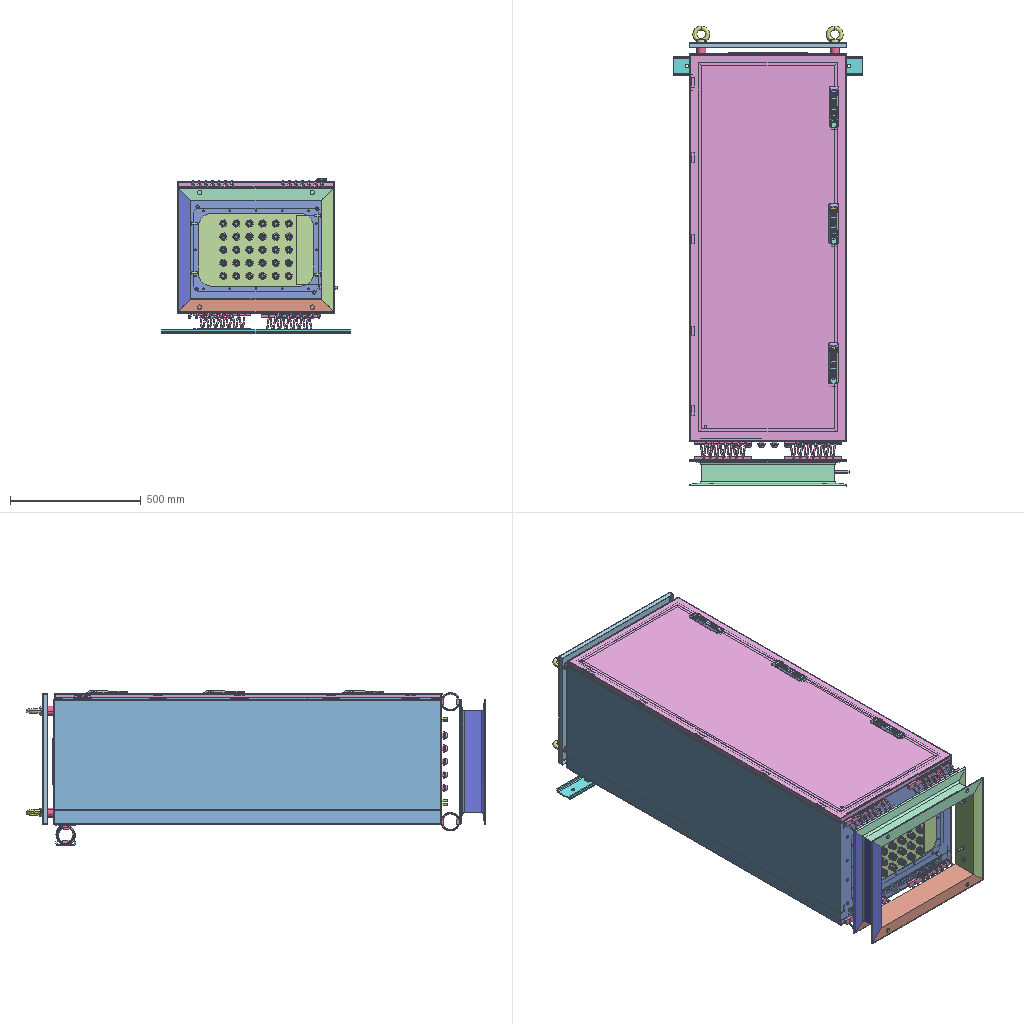Assembly | SolidWorks | 42 different items | 120 placed | box 720 x 1756 x 593 mm
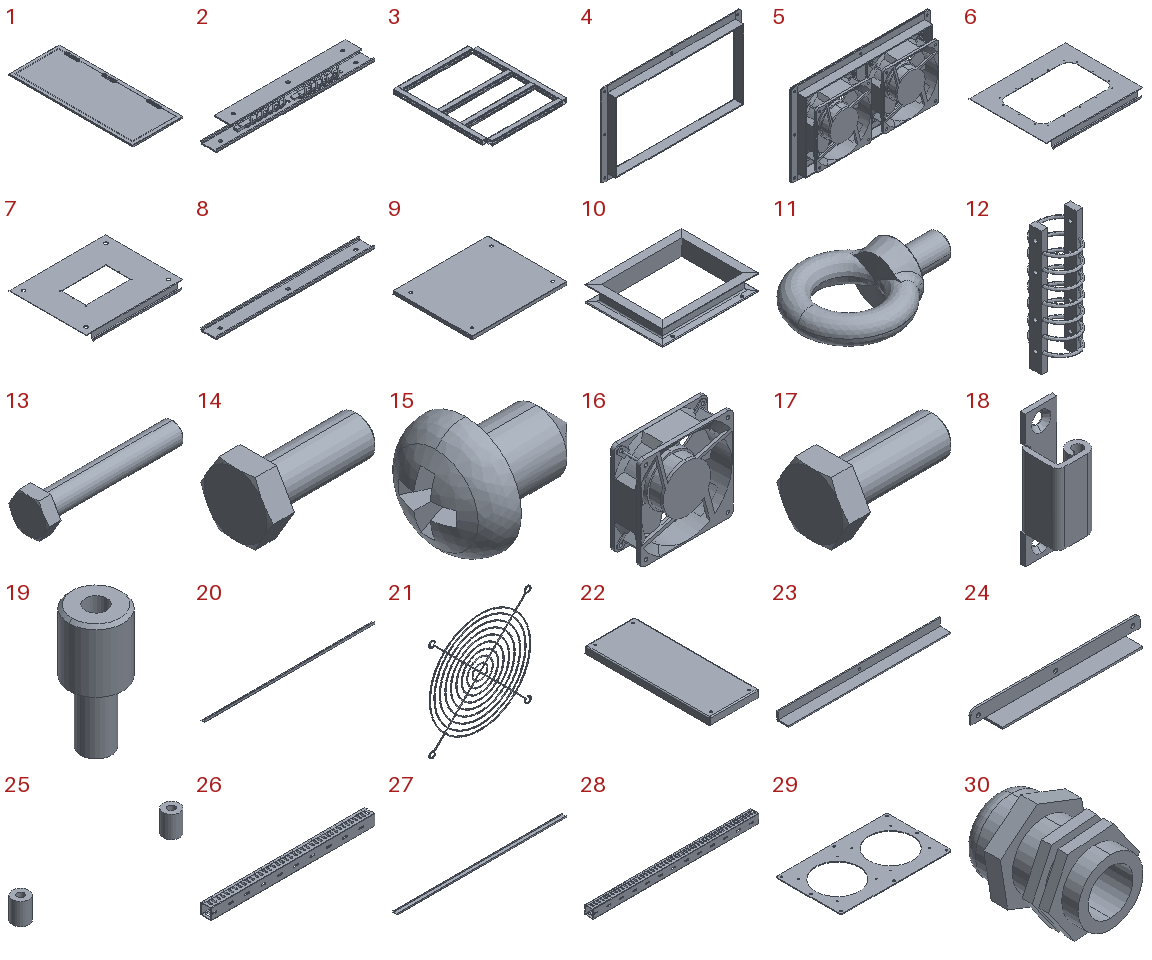Parts list (item | name | quantity | parent item | size | volume | features):
1 | (subassembly) | x1 | - | 599 x 1482 x 37.95 mm | 2644503 mm3 | -
2 | (subassembly) | x1 | - | 720 x 75 x 82.954 mm | 767649 mm3 | -
3 | (subassembly) | x1 | - | - | 575981 mm3 | -
4 | (subassembly) | x1 | in 5 | 300 x 20 x 176 mm | 55930 mm3 | -
5 | (subassembly) | x1 | - | 300 x 40.8 x 176 mm | 500898 mm3 | -
6 | - | x1 | - | 600 x 496 x 35 mm | 393982 mm3 | features MoveFace 2, BaseBody 1
7 | - | x1 | - | 600 x 496 x 35 mm | 549272 mm3 | features ICE 2, MoveFace 2, BaseBody 1
8 | - | x1 | in 2 | 720 x 75 x 15 mm | 322694 mm3 | features MoveFace 4, Fillet 2, BaseBody 1, ICE 1
9 | - | x1 | - | 600 x 500 x 20 mm | 675087 mm3 | features BaseBody 1, MoveFace 1
10 | - | x1 | - | 600 x 478 x 100 mm | 2451873 mm3 | features BaseBody 4, MoveCopyBody 2, MoveFace 2
11 | - | x4 | - | 91.2 x 64.4 x 35.09 mm | 39752 mm3 | features BaseBody 1
12 | - | x6 | in 2 | 71 x 70 x 216 mm | 111132 mm3 | features BaseBody 1, ICE 1
13 | - | x1 | - | 66.4 x 18.475 x 16 mm | 6099 mm3 | features BaseBody 1
14 | - | x1 | - | 18.975 x 11.258 x 9.75 mm | 741.836 mm3 | features BaseBody 1, MoveFace 1, Scale 1
15 | - | x6 | - | 14.243 x 11.05 x 11.056 mm | 485.827 mm3 | features BaseBody 1, MoveFace 1
16 | - | x2 | in 5 | 119.126 x 38.1 x 119.126 mm | 190423 mm3 | features BaseBody 1
17 | - | x8 | - | 25.3 x 15.011 x 13 mm | 1758 mm3 | features BaseBody 1, MoveFace 1
18 | - | x5 | - | 20 x 20 x 67 mm | 6811 mm3 | features BaseBody 1
19 | - | x4 | - | 35 x 35 x 80 mm | 47545 mm3 | features BaseBody 1
20 | - | x6 | - | 1472 x 31 x 20 mm | 172321 mm3 | features BaseBody 1, ICE 1, MoveFace 1
21 | - | x2 | in 5 | 111.7 x 0.7 x 111.7 mm | 1043 mm3 | features BaseBody 1
22 | - | x1 | - | 105 x 265 x 15 mm | 73841 mm3 | features BaseBody 1
23 | - | x2 | in 4 | 274 x 20 x 15 mm | 17798 mm3 | features BaseBody 1
24 | - | x2 | in 4 | 176 x 20 x 15 mm | 10168 mm3 | features BaseBody 1
25 | - | x2 | - | 122 x 12 x 16 mm | 3011 mm3 | features BaseBody 2
26 | - | x4 | in 3 | 502 x 31.5 x 34 mm | 88043 mm3 | features BaseBody 2, ICE 1
27 | - | x1 | - | 1475 x 40 x 12 mm | 174214 mm3 | features BaseBody 1, MoveFace 1
28 | - | x2 | in 3 | 640 x 31.5 x 34 mm | 111904 mm3 | features BaseBody 2
29 | - | x1 | in 5 | 300 x 176 x 2 mm | 62035 mm3 | features BaseBody 1
30 | - | x30 | - | 27.604 x 35 x 28.514 mm | 7936 mm3 | features ICE 5, Extrusion 1, Fillet 1, Shell 1
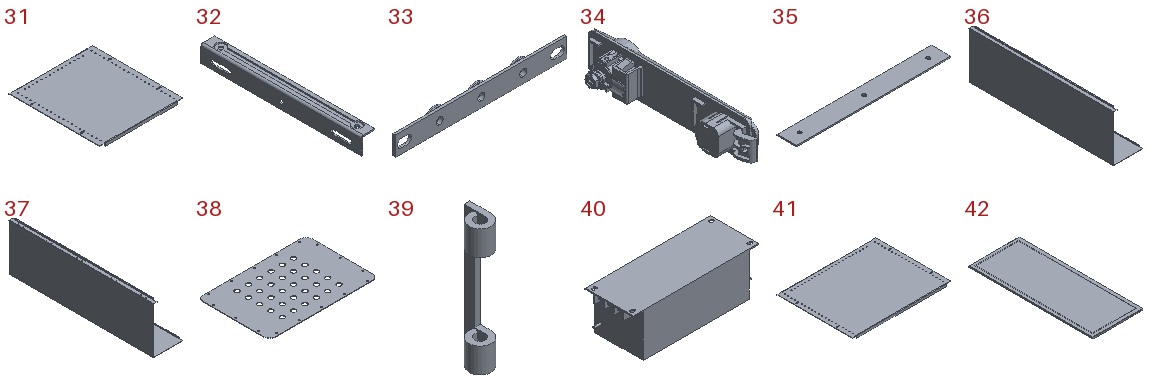31 | - | x6 | - | 406 x 440 x 15 mm | 372648 mm3 | features ICE 5, MoveFace 4, BaseBody 1
32 | - | x1 | - | 20 x 233 x 25 mm | 22029 mm3 | features ICE 4, Extrusion 1
33 | - | x2 | - | 123 x 4 x 15 mm | 4060 mm3 | features ICE 2, Extrusion 1
34 | - | x3 | in 1 | 37.95 x 165.2 x 36 mm | 54384 mm3 | features BaseBody 4
35 | - | x1 | in 2 | 600 x 75 x 5 mm | 222691 mm3 | features MoveFace 2, BaseBody 1
36 | - | x1 | - | 300 x 1476 x 496 mm | 2482636 mm3 | features ICE 3, MoveFace 3, BaseBody 1, Fillet 1
37 | - | x1 | - | 300 x 1476 x 496 mm | 2482160 mm3 | features MoveFace 6, ICE 3, BaseBody 1, Fillet 1
38 | - | x1 | - | 480 x 318 x 2 mm | 284296 mm3 | features ICE 2, BaseBody 1
39 | - | x1 | - | 10.6 x 15.5 x 60 mm | 2458 mm3 | features BaseBody 1
40 | - | x1 | - | 263 x 100 x 90 mm | 2010436 mm3 | features BaseBody 8
41 | - | x1 | - | 580 x 440 x 15 mm | 534266 mm3 | features ICE 4, MoveFace 2, BaseBody 1
42 | - | x1 | in 1 | 599 x 1482 x 20 mm | 2481350 mm3 | features ICE 6, MoveFace 6, BaseBody 1
Mates (type | each side: item.copy, entity, surface, feature):
In the top assembly
Coincident | 10.1 face plane Input 4 | 12.1 face plane Input 1 | 2 times
Coincident | 10.1 face plane Input 4 | 12.2 face plane Input 1 | 2 times
Coincident | 10.1 face plane Input 1 | 12.3 face plane Input 1 | 2 times
Coincident | 10.1 face plane Input 1 | 12.4 face plane Input 1 | 2 times
Coincident | 6.1 face plane Input 1 | 12.2 face plane Input 1 | 2 times
Coincident | 6.1 face plane Input 1 | 38.1 face plane Input 1
Concentric | 6.1 face cylinder Input 1 | 38.1 face cylinder Input 1 | 2 times
Coincident | 6.1 face plane Input 1 | 27.1 face plane Input 1
Coincident | 20.1 face plane Input 1 | 41.1 face plane Input 1
Coincident | 40.1 face plane Input 5 | 22.1 face plane Input 1
Concentric | 40.1 edge | 22.1 face cylinder Input 1
Concentric | 40.1 face cylinder Input 5 | 22.1 face cylinder Input 1
Coincident | 6.1 face plane Input 1 | 25.1 face plane Input 2
Coincident | 6.1 face plane Input 1 | 25.2 face plane Input 1
Concentric | 18.1 face cylinder Input 1 | 39.1 face cylinder Input 1
Coincident | 18.1 face plane Input 1 | 39.1 face plane Input 1
Coincident | 6.1 face plane Input 1 | 37.1 face plane Input 1 | 3 times
Coincident | 6.1 face plane Input 1 | 36.1 face plane Input 1 | 2 times
Coincident | 6.1 edge | 36.1 face plane Input 1
Coincident | 18.1 face plane Input 1 | 37.1 face plane Input 1
Concentric | 18.1 face cone Input 1 | 37.1 face cylinder Input 1 | 2 times
Coincident | 18.2 face plane Input 1 | 37.1 face plane Input 1
Concentric | 18.2 face cone Input 1 | 37.1 face cylinder Input 1 | 2 times
Coincident | 37.1 face plane Input 1 | 18.3 face plane Input 1
Concentric | 37.1 edge | 18.3 face cone Input 1 | 2 times
Coincident | 37.1 face plane Input 1 | 18.4 face plane Input 1
Concentric | 37.1 edge | 18.4 face cone Input 1 | 2 times
Coincident | 37.1 face plane Input 1 | 18.5 face plane Input 1
Concentric | 37.1 edge | 18.5 face cone Input 1
Concentric | 37.1 face cylinder Input 1 | 18.5 face cone Input 1
Coincident | 42.1 face plane Input 1 | 39.1 face plane Input 1 | 2 times
Parallel | 7.1 face plane Input 1 | 42.1 face plane Input 1
Coincident | 6.1 face plane Input 1 | 42.1 face plane Input 1
Concentric | 7.1 face cylinder Input 1 | 19.1 face cylinder Input 1
Coincident | 7.1 face plane Input 1 | 19.1 face plane Input 1
Concentric | 7.1 face cylinder Input 1 | 19.2 face cylinder Input 1
Coincident | 7.1 face plane Input 1 | 19.2 face plane Input 1
Concentric | 7.1 face cylinder Input 1 | 19.3 face cylinder Input 1
Coincident | 7.1 face plane Input 1 | 19.3 face plane Input 1
Concentric | 7.1 face cylinder Input 1 | 19.4 face cylinder Input 1
Coincident | 7.1 face plane Input 1 | 19.4 face plane Input 1
Coincident | 9.1 face plane Input 1 | 19.4 face plane Input 1
Concentric | 19.1 face cylinder Input 1 | 9.1 face cylinder Input 1
Concentric | 9.1 face cylinder Input 1 | 19.2 face cylinder Input 1
Concentric | 19.1 face cylinder Input 1 | 11.1 face cylinder Input 1
Coincident | 9.1 face plane Input 1 | 11.1 face plane Input 1
Concentric | 19.4 face cylinder Input 1 | 11.2 face cylinder Input 1
Coincident | 9.1 face plane Input 1 | 11.2 face plane Input 1
Concentric | 19.3 face cylinder Input 1 | 11.3 face cylinder Input 1
Coincident | 9.1 face plane Input 1 | 11.3 face plane Input 1
Concentric | 19.2 face cylinder Input 1 | 11.4 face cylinder Input 1
Coincident | 9.1 face plane Input 1 | 11.4 face plane Input 1
Coincident | 20.2 face plane Input 1 | 37.1 face plane Input 1
Coincident | 7.1 face plane Input 1 | 37.1 face plane Input 1 | 3 times
Coincident | assembly face | 37.1 face plane Input 1 | 2 times
Concentric | 7.1 face cylinder Cut-Extrude2 | 24.1 face cylinder Input 1
Concentric | 7.1 face cylinder Cut-Extrude2 | 23.1 face cylinder Input 1
Coincident | 7.1 face plane Input 1 | 24.1 face plane Input 1
Concentric | 38.1 face cylinder Cut-Extrude1 | 30.1 face cylinder Boss-Extrude1
Coincident | 38.1 face plane Input 1 | 30.1 face plane Boss-Extrude5
Coincident | 6.1 face plane Input 1 | 32.1 face plane Boss-Extrude1 | 2 times
Coincident | 10.1 face plane Input 3 | 13.1 face plane Input 1
Coincident | 10.1 face plane Input 2 | 17.1 face plane Input 1
Coincident | 10.1 face plane Input 2 | 17.2 face plane Input 1
Coincident | 10.1 face plane Input 3 | 17.3 face plane Input 1
Coincident | 10.1 face plane Input 3 | 17.4 face plane Input 1
Coincident | 38.1 face plane Input 1 | 17.5 face plane Input 1
Coincident | 38.1 face plane Input 1 | 17.6 face plane Input 1
Coincident | 38.1 face plane Input 1 | 17.7 face plane Input 1
Coincident | 38.1 face plane Input 1 | 17.8 face plane Input 1
Coincident | 25.1 face plane Input 1 | 33.1 face plane Boss-Extrude1
Slot | 25.1 face cylinder Input 1 | 33.1 face plane Boss-Extrude1
Slot | 25.1 face cylinder Input 2 | 33.1 face plane Boss-Extrude1
Coincident | 25.2 face plane Input 1 | 33.2 face plane Boss-Extrude1
Slot | 33.2 face plane Boss-Extrude1 | 25.2 face cylinder Input 2
Slot | 33.2 face plane Boss-Extrude1 | 25.2 face cylinder Input 1
Concentric | 33.1 face cylinder Boss-Extrude1 | 15.1 face cylinder Input 1
Coincident | 33.1 face plane Boss-Extrude3 | 15.1 face plane Input 1
Concentric | 33.1 face cylinder Boss-Extrude1 | 15.2 face cylinder Input 1
Coincident | 33.1 face plane Boss-Extrude3 | 15.2 face plane Input 1
Concentric | 33.1 face cylinder Boss-Extrude1 | 15.3 face cylinder Input 1
Coincident | 33.1 face plane Boss-Extrude3 | 15.3 face plane Input 1
Concentric | 33.2 face cylinder Boss-Extrude1 | 15.4 face cylinder Input 1
Coincident | 33.2 face plane Boss-Extrude3 | 15.4 face plane Input 1
Concentric | 33.2 face cylinder Boss-Extrude1 | 15.5 face cylinder Input 1
Coincident | 33.2 face plane Boss-Extrude3 | 15.5 face plane Input 1
Concentric | 33.2 face cylinder Boss-Extrude1 | 15.6 face cylinder Input 1
Coincident | 33.2 face plane Boss-Extrude3 | 15.6 face plane Input 1
Coincident | 6.1 face plane Input 1 | 26.1 face plane Input 1
Coincident | 20.2 face plane Input 1 | 28.1 face plane Input 1
Coincident | 6.1 face plane Input 1 | 20.3 face plane Input 1
Coincident | 28.1 face plane Input 2 | 20.3 face plane Input 1
Coincident | 37.1 face plane Input 1 | 20.3 edge
Coincident | 6.1 face plane Input 1 | 20.4 face plane Cut-Extrude1
Coincident | 37.1 face plane Input 1 | 20.4 face plane Input 1
Coincident | 37.1 edge | 20.4 face plane Input 1
Coincident | 20.4 face plane Input 1 | 31.1 face plane Input 1
Parallel | 37.1 face plane Input 1 | 31.1 face plane Input 1
Coincident | 20.4 face plane Input 1 | 31.2 face plane Input 1
Parallel | 37.1 face plane Input 1 | 31.2 face plane Input 1
Coincident | 20.4 face plane Input 1 | 31.3 face plane Input 1
Parallel | 37.1 face plane Input 1 | 31.3 face plane Input 1
Coincident | 6.1 face plane Input 1 | 20.5 face plane Cut-Extrude1
Coincident | 28.2 face plane Input 2 | 20.5 face plane Input 1
Coincident | 36.1 face plane Input 1 | 20.5 face plane Input 1
Coincident | 6.1 face plane Input 1 | 20.6 face plane Input 1
Coincident | 36.1 face plane Input 1 | 20.6 face plane Input 1
Coincident | 36.1 edge | 20.6 face plane Input 1
Coincident | 20.6 face plane Input 1 | 31.4 face plane Input 1
Parallel | 36.1 face plane Input 1 | 31.4 face plane Input 1
Coincident | 20.6 face plane Input 1 | 31.5 face plane Input 1
Parallel | 36.1 face plane Input 1 | 31.5 face plane Input 1
Coincident | 20.6 face plane Input 1 | 31.6 face plane Input 1
Parallel | 36.1 face plane Input 1 | 31.6 face plane Input 1
Coincident | 38.1 face plane Input 1 | 22.1 face plane Input 1
Coincident | 31.1 face plane Input 1 | 31.2 face plane Input 1 | 2 times
Coincident | 31.2 face plane Input 1 | 31.3 face plane Input 1 | 2 times
Coincident | 31.4 face plane Input 1 | 31.5 face plane Input 1 | 2 times
Coincident | 31.5 face plane Input 1 | 31.6 face plane Input 1 | 2 times
Slot | 31.1 face cylinder Input 1 | 20.4 face cylinder Input 1
Slot | 31.4 face cylinder Input 1 | 20.6 face cylinder Input 1
Coincident | 42.1 face plane Input 1 | 14.1 face plane Input 1
In subassembly 1
Coincident | 42.2 face plane Input 1 | 34.1 face plane Input 3
Coincident | 42.2 face plane Input 1 | 34.2 face plane Input 3
Coincident | 34.1 face plane Input 3 | 34.2 face plane Input 3
Coincident | 42.2 face plane Input 1 | 34.3 face plane Input 3
Coincident | 34.1 face plane Input 3 | 34.3 face plane Input 3
In subassembly 2
Coincident | 12.1 face plane Input 1 | 35.1 face plane Input 1
Coincident | 8.1 face plane Input 1 | 35.1 face plane Input 1
DistanceDim | 35.1 face plane Input 1 | 8.1 face plane Input 1